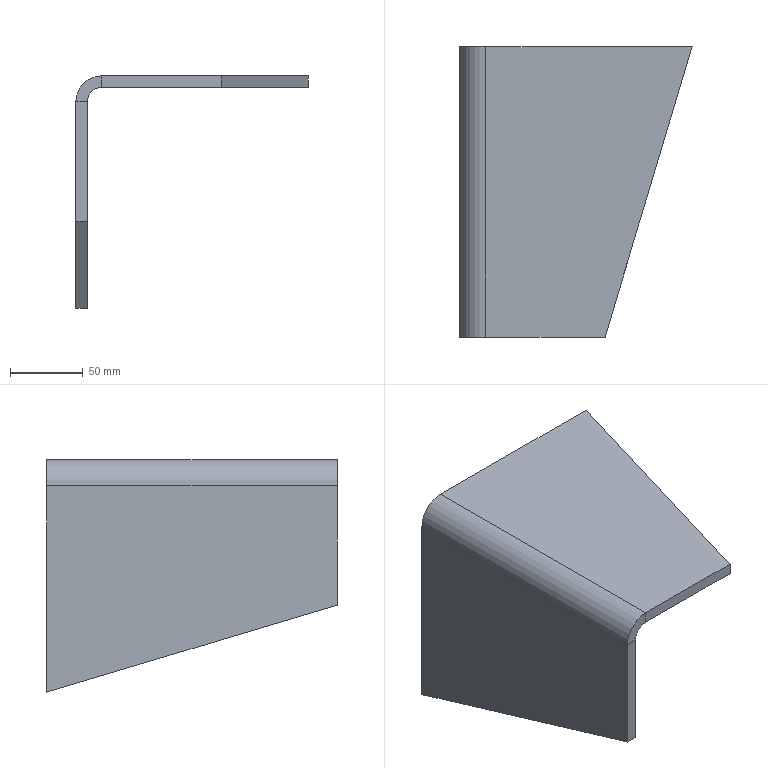Part | SolidWorks | features Fillet 2, ICE 2, EdgeFlange 1, FlatPattern 1, SMBaseFlange 1, SheetMetal 1 | 1 solid | 14 faces | box 160 x 200 x 160 mm | volume 393586 mm3 | plane 12 | cylinder 2 | commonest cylinder face diameters 20 x1 36 x1
STEP:
#1=CARTESIAN_POINT('',(92.,0.,0.));
#2=VERTEX_POINT('',#1);
#3=CARTESIAN_POINT('',(92.,0.,8.));
#4=VERTEX_POINT('',#3);
#5=CARTESIAN_POINT('',(92.,0.,0.));
#6=DIRECTION('',(0.,0.,1.));
#7=VECTOR('',#6,1000.);
#8=LINE('',#5,#7);
#9=EDGE_CURVE('',#2,#4,#8,.T.);
#10=ORIENTED_EDGE('',*,*,#9,.T.);
#11=CARTESIAN_POINT('',(10.,0.,8.));
#12=VERTEX_POINT('',#11);
#13=CARTESIAN_POINT('',(152.,0.,8.));
#14=DIRECTION('',(1.,0.,0.));
#15=VECTOR('',#14,1000.);
#16=LINE('',#13,#15);
#17=EDGE_CURVE('',#12,#4,#16,.T.);
#18=ORIENTED_EDGE('',*,*,#17,.F.);
#19=CARTESIAN_POINT('',(10.,0.,0.));
#20=VERTEX_POINT('',#19);
#21=CARTESIAN_POINT('',(10.,0.,0.));
#22=DIRECTION('',(0.,0.,1.));
#23=VECTOR('',#22,1000.);
#24=LINE('',#21,#23);
#25=EDGE_CURVE('',#20,#12,#24,.T.);
#26=ORIENTED_EDGE('',*,*,#25,.F.);
#27=CARTESIAN_POINT('',(152.,0.,0.));
#28=DIRECTION('',(1.,0.,0.));
#29=VECTOR('',#28,1000.);
#30=LINE('',#27,#29);
#31=EDGE_CURVE('',#20,#2,#30,.T.);
#32=ORIENTED_EDGE('',*,*,#31,.T.);
#33=EDGE_LOOP('',(#10,#18,#26,#32));
#34=FACE_OUTER_BOUND('',#33,.T.);
#35=CARTESIAN_POINT('',(152.,0.,8.));
#36=DIRECTION('',(0.,1.,0.));
#37=DIRECTION('',(0.,0.,1.));
#38=AXIS2_PLACEMENT_3D('',#35,#36,#37);
#39=PLANE('',#38);
#40=ADVANCED_FACE('',(#34),#39,.F.);
#41=CARTESIAN_POINT('',(152.,200.,8.));
#42=VERTEX_POINT('',#41);
#43=CARTESIAN_POINT('',(84.404,-25.321,8.));
#44=DIRECTION('',(0.2873,0.9578,0.));
#45=VECTOR('',#44,1000.);
#46=LINE('',#43,#45);
#47=EDGE_CURVE('',#4,#42,#46,.T.);
#48=ORIENTED_EDGE('',*,*,#47,.T.);
#49=CARTESIAN_POINT('',(10.,200.,8.));
#50=VERTEX_POINT('',#49);
#51=CARTESIAN_POINT('',(0.,200.,8.));
#52=DIRECTION('',(-1.,0.,0.));
#53=VECTOR('',#52,1000.);
#54=LINE('',#51,#53);
#55=EDGE_CURVE('',#42,#50,#54,.T.);
#56=ORIENTED_EDGE('',*,*,#55,.T.);
#57=CARTESIAN_POINT('',(10.,0.,8.));
#58=DIRECTION('',(0.,1.,0.));
#59=VECTOR('',#58,1000.);
#60=LINE('',#57,#59);
#61=EDGE_CURVE('',#12,#50,#60,.T.);
#62=ORIENTED_EDGE('',*,*,#61,.F.);
#63=ORIENTED_EDGE('',*,*,#17,.T.);
#64=EDGE_LOOP('',(#48,#56,#62,#63));
#65=FACE_OUTER_BOUND('',#64,.T.);
#66=CARTESIAN_POINT('',(0.,0.,8.));
#67=DIRECTION('',(0.,0.,-1.));
#68=DIRECTION('',(-1.,0.,0.));
#69=AXIS2_PLACEMENT_3D('',#66,#67,#68);
#70=PLANE('',#69);
#71=ADVANCED_FACE('',(#65),#70,.F.);
#72=CARTESIAN_POINT('',(152.,200.,0.));
#73=VERTEX_POINT('',#72);
#74=CARTESIAN_POINT('',(10.,200.,0.));
#75=VERTEX_POINT('',#74);
#76=CARTESIAN_POINT('',(0.,200.,0.));
#77=DIRECTION('',(-1.,0.,0.));
#78=VECTOR('',#77,1000.);
#79=LINE('',#76,#78);
#80=EDGE_CURVE('',#73,#75,#79,.T.);
#81=ORIENTED_EDGE('',*,*,#80,.F.);
#82=CARTESIAN_POINT('',(84.404,-25.321,0.));
#83=DIRECTION('',(0.2873,0.9578,0.));
#84=VECTOR('',#83,1000.);
#85=LINE('',#82,#84);
#86=EDGE_CURVE('',#2,#73,#85,.T.);
#87=ORIENTED_EDGE('',*,*,#86,.F.);
#88=ORIENTED_EDGE('',*,*,#31,.F.);
#89=CARTESIAN_POINT('',(10.,200.,0.));
#90=DIRECTION('',(0.,-1.,0.));
#91=VECTOR('',#90,1000.);
#92=LINE('',#89,#91);
#93=EDGE_CURVE('',#75,#20,#92,.T.);
#94=ORIENTED_EDGE('',*,*,#93,.F.);
#95=EDGE_LOOP('',(#81,#87,#88,#94));
#96=FACE_OUTER_BOUND('',#95,.T.);
#97=CARTESIAN_POINT('',(0.,0.,0.));
#98=DIRECTION('',(0.,0.,-1.));
#99=DIRECTION('',(-1.,0.,0.));
#100=AXIS2_PLACEMENT_3D('',#97,#98,#99);
#101=PLANE('',#100);
#102=ADVANCED_FACE('',(#96),#101,.T.);
#103=CARTESIAN_POINT('',(0.,0.,-10.));
#104=VERTEX_POINT('',#103);
#105=CARTESIAN_POINT('',(0.,0.,-92.));
#106=VERTEX_POINT('',#105);
#107=CARTESIAN_POINT('',(0.,0.,0.));
#108=DIRECTION('',(0.,0.,-1.));
#109=VECTOR('',#108,1000.);
#110=LINE('',#107,#109);
#111=EDGE_CURVE('',#104,#106,#110,.T.);
#112=ORIENTED_EDGE('',*,*,#111,.F.);
#113=CARTESIAN_POINT('',(-8.,0.,-10.));
#114=VERTEX_POINT('',#113);
#115=CARTESIAN_POINT('',(0.,0.,-10.));
#116=DIRECTION('',(-1.,0.,0.));
#117=VECTOR('',#116,1000.);
#118=LINE('',#115,#117);
#119=EDGE_CURVE('',#104,#114,#118,.T.);
#120=ORIENTED_EDGE('',*,*,#119,.T.);
#121=CARTESIAN_POINT('',(-8.,0.,-92.));
#122=VERTEX_POINT('',#121);
#123=CARTESIAN_POINT('',(-8.,0.,0.));
#124=DIRECTION('',(0.,0.,-1.));
#125=VECTOR('',#124,1000.);
#126=LINE('',#123,#125);
#127=EDGE_CURVE('',#114,#122,#126,.T.);
#128=ORIENTED_EDGE('',*,*,#127,.T.);
#129=CARTESIAN_POINT('',(-8.,0.,-92.));
#130=DIRECTION('',(1.,0.,0.));
#131=VECTOR('',#130,1000.);
#132=LINE('',#129,#131);
#133=EDGE_CURVE('',#122,#106,#132,.T.);
#134=ORIENTED_EDGE('',*,*,#133,.T.);
#135=EDGE_LOOP('',(#112,#120,#128,#134));
#136=FACE_OUTER_BOUND('',#135,.T.);
#137=CARTESIAN_POINT('',(-8.,0.,0.));
#138=DIRECTION('',(0.,-1.,0.));
#139=DIRECTION('',(0.,0.,-1.));
#140=AXIS2_PLACEMENT_3D('',#137,#138,#139);
#141=PLANE('',#140);
#142=ADVANCED_FACE('',(#136),#141,.T.);
#143=CARTESIAN_POINT('',(-8.,200.,-10.));
#144=VERTEX_POINT('',#143);
#145=CARTESIAN_POINT('',(-8.,0.,-10.));
#146=DIRECTION('',(0.,1.,0.));
#147=VECTOR('',#146,1000.);
#148=LINE('',#145,#147);
#149=EDGE_CURVE('',#114,#144,#148,.T.);
#150=ORIENTED_EDGE('',*,*,#149,.T.);
#151=CARTESIAN_POINT('',(-8.,200.,-152.));
#152=VERTEX_POINT('',#151);
#153=CARTESIAN_POINT('',(-8.,200.,-152.));
#154=DIRECTION('',(0.,0.,1.));
#155=VECTOR('',#154,1000.);
#156=LINE('',#153,#155);
#157=EDGE_CURVE('',#152,#144,#156,.T.);
#158=ORIENTED_EDGE('',*,*,#157,.F.);
#159=CARTESIAN_POINT('',(-8.,200.,-152.));
#160=DIRECTION('',(0.,0.9578,-0.2873));
#161=VECTOR('',#160,1000.);
#162=LINE('',#159,#161);
#163=EDGE_CURVE('',#122,#152,#162,.T.);
#164=ORIENTED_EDGE('',*,*,#163,.F.);
#165=ORIENTED_EDGE('',*,*,#127,.F.);
#166=EDGE_LOOP('',(#150,#158,#164,#165));
#167=FACE_OUTER_BOUND('',#166,.T.);
#168=CARTESIAN_POINT('',(-8.,0.,0.));
#169=DIRECTION('',(1.,0.,0.));
#170=DIRECTION('',(0.,0.,-1.));
#171=AXIS2_PLACEMENT_3D('',#168,#169,#170);
#172=PLANE('',#171);
#173=ADVANCED_FACE('',(#167),#172,.F.);
#174=CARTESIAN_POINT('',(0.,200.,-152.));
#175=VERTEX_POINT('',#174);
#176=CARTESIAN_POINT('',(0.,200.,-10.));
#177=VERTEX_POINT('',#176);
#178=CARTESIAN_POINT('',(0.,200.,-152.));
#179=DIRECTION('',(0.,0.,1.));
#180=VECTOR('',#179,1000.);
#181=LINE('',#178,#180);
#182=EDGE_CURVE('',#175,#177,#181,.T.);
#183=ORIENTED_EDGE('',*,*,#182,.T.);
#184=CARTESIAN_POINT('',(0.,0.,-10.));
#185=DIRECTION('',(0.,1.,0.));
#186=VECTOR('',#185,1000.);
#187=LINE('',#184,#186);
#188=EDGE_CURVE('',#104,#177,#187,.T.);
#189=ORIENTED_EDGE('',*,*,#188,.F.);
#190=ORIENTED_EDGE('',*,*,#111,.T.);
#191=CARTESIAN_POINT('',(0.,200.,-152.));
#192=DIRECTION('',(0.,0.9578,-0.2873));
#193=VECTOR('',#192,1000.);
#194=LINE('',#191,#193);
#195=EDGE_CURVE('',#106,#175,#194,.T.);
#196=ORIENTED_EDGE('',*,*,#195,.T.);
#197=EDGE_LOOP('',(#183,#189,#190,#196));
#198=FACE_OUTER_BOUND('',#197,.T.);
#199=CARTESIAN_POINT('',(0.,0.,0.));
#200=DIRECTION('',(1.,0.,0.));
#201=DIRECTION('',(0.,0.,-1.));
#202=AXIS2_PLACEMENT_3D('',#199,#200,#201);
#203=PLANE('',#202);
#204=ADVANCED_FACE('',(#198),#203,.T.);
#205=CARTESIAN_POINT('',(0.,200.,-10.));
#206=DIRECTION('',(-1.,0.,0.));
#207=VECTOR('',#206,1000.);
#208=LINE('',#205,#207);
#209=EDGE_CURVE('',#177,#144,#208,.T.);
#210=ORIENTED_EDGE('',*,*,#209,.F.);
#211=ORIENTED_EDGE('',*,*,#182,.F.);
#212=CARTESIAN_POINT('',(-8.,200.,-152.));
#213=DIRECTION('',(1.,0.,0.));
#214=VECTOR('',#213,1000.);
#215=LINE('',#212,#214);
#216=EDGE_CURVE('',#152,#175,#215,.T.);
#217=ORIENTED_EDGE('',*,*,#216,.F.);
#218=ORIENTED_EDGE('',*,*,#157,.T.);
#219=EDGE_LOOP('',(#210,#211,#217,#218));
#220=FACE_OUTER_BOUND('',#219,.T.);
#221=CARTESIAN_POINT('',(-8.,200.,-152.));
#222=DIRECTION('',(0.,1.,0.));
#223=DIRECTION('',(0.,0.,1.));
#224=AXIS2_PLACEMENT_3D('',#221,#222,#223);
#225=PLANE('',#224);
#226=ADVANCED_FACE('',(#220),#225,.T.);
#227=ORIENTED_EDGE('',*,*,#195,.F.);
#228=ORIENTED_EDGE('',*,*,#133,.F.);
#229=ORIENTED_EDGE('',*,*,#163,.T.);
#230=ORIENTED_EDGE('',*,*,#216,.T.);
#231=EDGE_LOOP('',(#227,#228,#229,#230));
#232=FACE_OUTER_BOUND('',#231,.T.);
#233=CARTESIAN_POINT('',(-8.,200.,-152.));
#234=DIRECTION('',(0.,-0.2873,-0.9578));
#235=DIRECTION('',(0.,0.9578,-0.2873));
#236=AXIS2_PLACEMENT_3D('',#233,#234,#235);
#237=PLANE('',#236);
#238=ADVANCED_FACE('',(#232),#237,.T.);
#239=CARTESIAN_POINT('',(10.,200.,0.));
#240=DIRECTION('',(0.,0.,1.));
#241=VECTOR('',#240,1000.);
#242=LINE('',#239,#241);
#243=EDGE_CURVE('',#75,#50,#242,.T.);
#244=ORIENTED_EDGE('',*,*,#243,.F.);
#245=CARTESIAN_POINT('',(10.,200.,-10.));
#246=DIRECTION('',(0.,1.,0.));
#247=DIRECTION('',(0.,0.,-1.));
#248=AXIS2_PLACEMENT_3D('',#245,#246,#247);
#249=CIRCLE('',#248,10.);
#250=EDGE_CURVE('',#177,#75,#249,.T.);
#251=ORIENTED_EDGE('',*,*,#250,.F.);
#252=ORIENTED_EDGE('',*,*,#209,.T.);
#253=CARTESIAN_POINT('',(10.,200.,-10.));
#254=DIRECTION('',(0.,1.,0.));
#255=DIRECTION('',(0.,0.,-1.));
#256=AXIS2_PLACEMENT_3D('',#253,#254,#255);
#257=CIRCLE('',#256,18.);
#258=EDGE_CURVE('',#144,#50,#257,.T.);
#259=ORIENTED_EDGE('',*,*,#258,.T.);
#260=EDGE_LOOP('',(#244,#251,#252,#259));
#261=FACE_OUTER_BOUND('',#260,.T.);
#262=CARTESIAN_POINT('',(10.,200.,-10.));
#263=DIRECTION('',(0.,1.,0.));
#264=DIRECTION('',(0.,0.,1.));
#265=AXIS2_PLACEMENT_3D('',#262,#263,#264);
#266=PLANE('',#265);
#267=ADVANCED_FACE('',(#261),#266,.T.);
#268=CARTESIAN_POINT('',(10.,0.,-10.));
#269=DIRECTION('',(0.,-1.,0.));
#270=DIRECTION('',(0.,0.,-1.));
#271=AXIS2_PLACEMENT_3D('',#268,#269,#270);
#272=CIRCLE('',#271,10.);
#273=EDGE_CURVE('',#20,#104,#272,.T.);
#274=ORIENTED_EDGE('',*,*,#273,.F.);
#275=ORIENTED_EDGE('',*,*,#25,.T.);
#276=CARTESIAN_POINT('',(10.,0.,-10.));
#277=DIRECTION('',(0.,-1.,0.));
#278=DIRECTION('',(0.,0.,-1.));
#279=AXIS2_PLACEMENT_3D('',#276,#277,#278);
#280=CIRCLE('',#279,18.);
#281=EDGE_CURVE('',#12,#114,#280,.T.);
#282=ORIENTED_EDGE('',*,*,#281,.T.);
#283=ORIENTED_EDGE('',*,*,#119,.F.);
#284=EDGE_LOOP('',(#274,#275,#282,#283));
#285=FACE_OUTER_BOUND('',#284,.T.);
#286=CARTESIAN_POINT('',(10.,0.,-10.));
#287=DIRECTION('',(0.,1.,0.));
#288=DIRECTION('',(0.,0.,1.));
#289=AXIS2_PLACEMENT_3D('',#286,#287,#288);
#290=PLANE('',#289);
#291=ADVANCED_FACE('',(#285),#290,.F.);
#292=ORIENTED_EDGE('',*,*,#149,.F.);
#293=ORIENTED_EDGE('',*,*,#281,.F.);
#294=ORIENTED_EDGE('',*,*,#61,.T.);
#295=ORIENTED_EDGE('',*,*,#258,.F.);
#296=EDGE_LOOP('',(#292,#293,#294,#295));
#297=FACE_OUTER_BOUND('',#296,.T.);
#298=CARTESIAN_POINT('',(10.,0.,-10.));
#299=DIRECTION('',(0.,-1.,0.));
#300=DIRECTION('',(0.,0.,1.));
#301=AXIS2_PLACEMENT_3D('',#298,#299,#300);
#302=CYLINDRICAL_SURFACE('',#301,18.);
#303=ADVANCED_FACE('',(#297),#302,.T.);
#304=ORIENTED_EDGE('',*,*,#188,.T.);
#305=ORIENTED_EDGE('',*,*,#250,.T.);
#306=ORIENTED_EDGE('',*,*,#93,.T.);
#307=ORIENTED_EDGE('',*,*,#273,.T.);
#308=EDGE_LOOP('',(#304,#305,#306,#307));
#309=FACE_OUTER_BOUND('',#308,.T.);
#310=CARTESIAN_POINT('',(10.,0.,-10.));
#311=DIRECTION('',(0.,-1.,0.));
#312=DIRECTION('',(0.,0.,1.));
#313=AXIS2_PLACEMENT_3D('',#310,#311,#312);
#314=CYLINDRICAL_SURFACE('',#313,10.);
#315=ADVANCED_FACE('',(#309),#314,.F.);
#316=ORIENTED_EDGE('',*,*,#243,.T.);
#317=ORIENTED_EDGE('',*,*,#55,.F.);
#318=CARTESIAN_POINT('',(152.,200.,8.));
#319=DIRECTION('',(0.,0.,-1.));
#320=VECTOR('',#319,1000.);
#321=LINE('',#318,#320);
#322=EDGE_CURVE('',#42,#73,#321,.T.);
#323=ORIENTED_EDGE('',*,*,#322,.T.);
#324=ORIENTED_EDGE('',*,*,#80,.T.);
#325=EDGE_LOOP('',(#316,#317,#323,#324));
#326=FACE_OUTER_BOUND('',#325,.T.);
#327=CARTESIAN_POINT('',(0.,200.,8.));
#328=DIRECTION('',(0.,-1.,0.));
#329=DIRECTION('',(0.,0.,-1.));
#330=AXIS2_PLACEMENT_3D('',#327,#328,#329);
#331=PLANE('',#330);
#332=ADVANCED_FACE('',(#326),#331,.F.);
#333=ORIENTED_EDGE('',*,*,#86,.T.);
#334=ORIENTED_EDGE('',*,*,#322,.F.);
#335=ORIENTED_EDGE('',*,*,#47,.F.);
#336=ORIENTED_EDGE('',*,*,#9,.F.);
#337=EDGE_LOOP('',(#333,#334,#335,#336));
#338=FACE_OUTER_BOUND('',#337,.T.);
#339=CARTESIAN_POINT('',(84.404,-25.321,0.));
#340=DIRECTION('',(-0.9578,0.2873,0.));
#341=DIRECTION('',(0.2873,0.9578,0.));
#342=AXIS2_PLACEMENT_3D('',#339,#340,#341);
#343=PLANE('',#342);
#344=ADVANCED_FACE('',(#338),#343,.F.);
#345=CLOSED_SHELL('',(#40,#71,#102,#142,#173,#204,#226,#238,#267,#291,#303,#315,#332,#344));
#346=MANIFOLD_SOLID_BREP('',#345);
#347=CARTESIAN_POINT('',(0.,0.,0.));
#348=DIRECTION('',(0.,0.,1.));
#349=DIRECTION('',(1.,0.,0.));
#350=AXIS2_PLACEMENT_3D('',#347,#348,#349);
#351=(LENGTH_UNIT()NAMED_UNIT(*)SI_UNIT(.MILLI.,.METRE.));
#352=UNCERTAINTY_MEASURE_WITH_UNIT(LENGTH_MEASURE(0.00001),#351,'','');
#353=(NAMED_UNIT(*)PLANE_ANGLE_UNIT()SI_UNIT($,.RADIAN.));
#354=(NAMED_UNIT(*)SI_UNIT($,.STERADIAN.)SOLID_ANGLE_UNIT());
#355=(GEOMETRIC_REPRESENTATION_CONTEXT(3)GLOBAL_UNCERTAINTY_ASSIGNED_CONTEXT((#352))GLOBAL_UNIT_ASSIGNED_CONTEXT((#351,#353,#354))REPRESENTATION_CONTEXT('',''));
#356=ADVANCED_BREP_SHAPE_REPRESENTATION('',(#346,#350),#355);